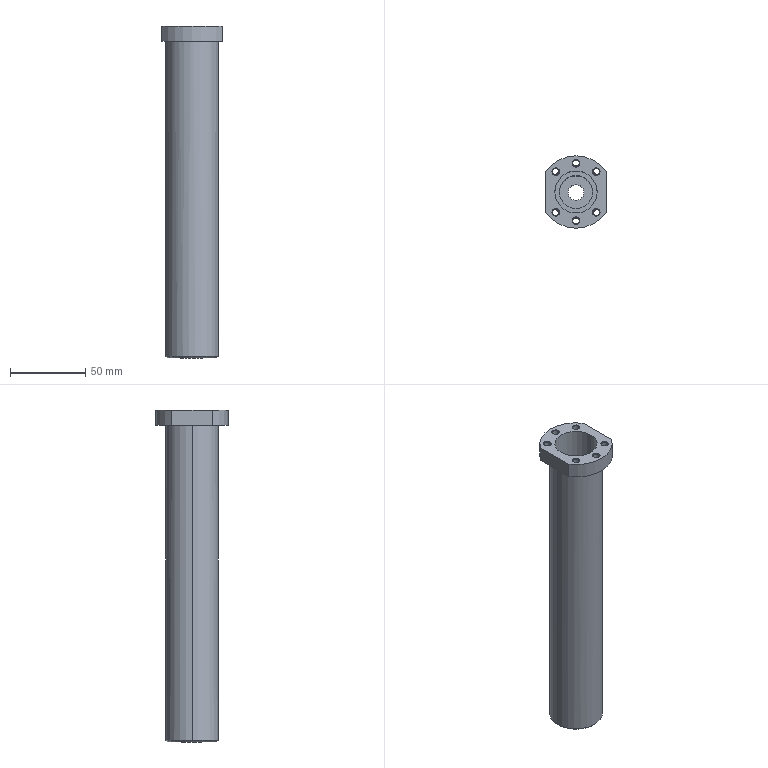Part | SolidWorks | features BaseBody 1 | 1 solid | 51 faces | box 40 x 48 x 220 mm | volume 131790 mm3 | cylinder 22 | cone 22 | plane 7 | commonest cylinder face diameters 4.2 x12 10.5 x2 22 x2 28 x2 35 x2 48 x2